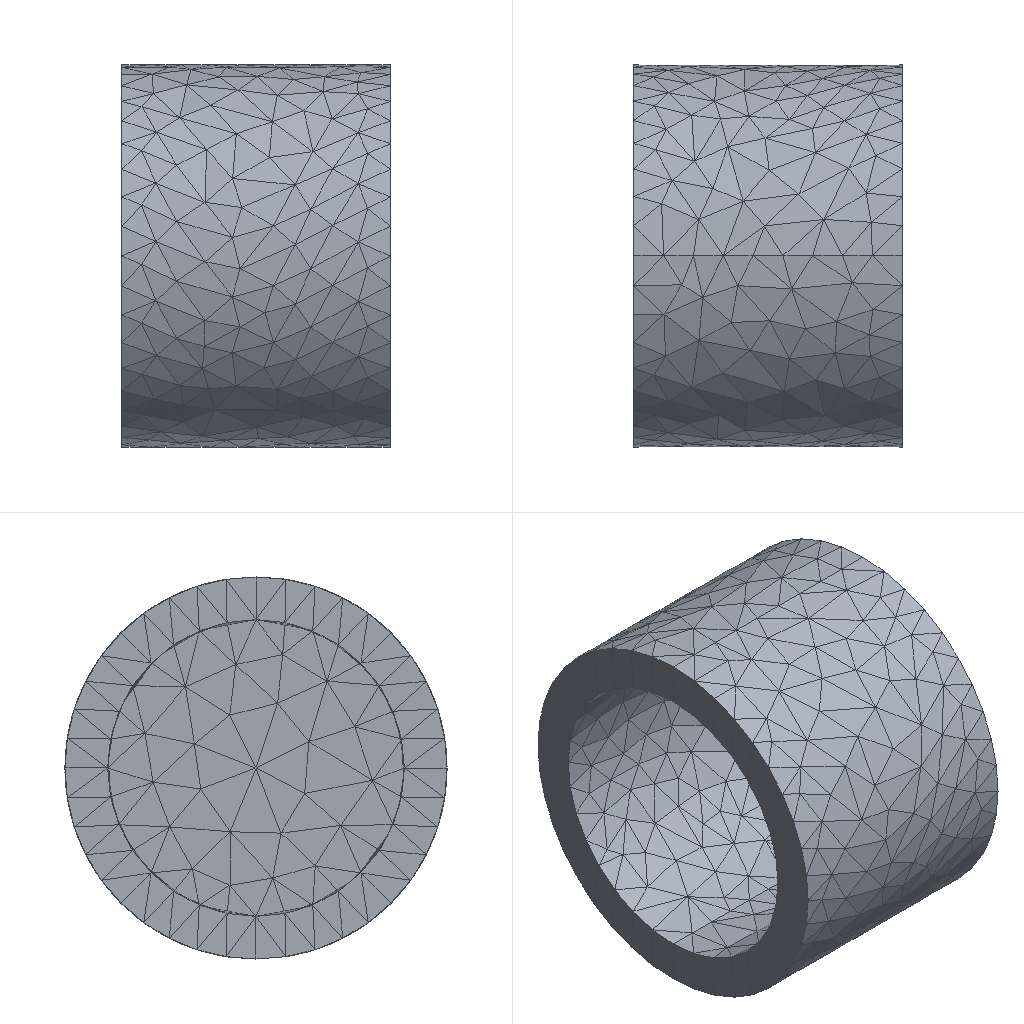Simulation study | ansys workbench
Ansys APDL input file, long lists of numbers shortened:
/batch
/config,noeldb,1     ! force off writing results to database
*get,_wallstrt,active,,time,wall
! ANSYS input file written by Workbench version 2022 R1
! File used for geometry attach:
/title,wbnew--____ (A5)
! ****** Begin Custom Load Command Snippet ******
/COM, ACT Extensions:
/COM,     LSDYNA, 2021.1
/COM,
! ****** End   Custom Load Command Snippet ******
*DIM,_wb_ProjectScratch_dir,string,248
_wb_ProjectScratch_dir(1) = ''
*DIM,_wb_SolverFiles_dir,string,248
_wb_SolverFiles_dir(1) = ''
*DIM,_wb_userfiles_dir,string,248
_wb_userfiles_dir(1) = ''
/com,--- Data in consistent NMM units. See Solving Units in the help system for more information.
/units,MPA
/nopr
/wb,file,start              !  signify a WB generated input file
/prep7
! Turn off shape checking because checks already performed inside WB mesher.
! See help system for more information.
SHPP,OFF,,NOWARN
/nolist
etcon,set             ! allow ANSYS to choose best KEYOP's for 180x elements, resets any applicable keyopt to MAPDL defaults
/com,*********** Nodes for the whole assembly ***********
nblock,3,,4614
(1i9,3e20.9e3)
        1     1.305000000E+03     0.000000000E+00     1.789968367E+02
! (4194 more lines like these left out)
-1
/wb,elem,start            !  set before creation of elements
/com,*********** Elements for Body 1 "__1-FreeParts|__-__1" ***********
et,1,187
eblock,19,solid,,2247
(19i9)
        1        1        1        1        0        0        0        0       10        0        1      105      684      200      612     1448     1992     1440     1445
! (4493 more lines like these left out)
-1
/wb,elem,end               !  done creating elements
/com,*********** Send User Defined Coordinate System(s) ***********
csys,0
toffst,273.15,  ! Temperature offset from absolute zero
/com,*********** Set Reference Temperature ***********
tref,22.
/wb,mat,start              !  starting to send materials
/com,*********** Send Materials ***********
Temperature = 'TEMP' ! Temperature
MP,DENS,1,7.85e-09,	! tonne mm^-3
MP,ALPX,1,1.2e-05,	! C^-1
MP,C,1,434000000,	! mm^2 s^-2 C^-1
MP,KXX,1,60.5,	! tonne mm s^-3 C^-1
MP,RSVX,1,0.00017,	! ohm mm
MP,EX,1,200000,	! tonne s^-2 mm^-1
MP,NUXY,1,0.3,
MP,MURX,1,10000,
/wb,mat,end                !  done sending materials
!************************* Model Summary ********************
!__1-FreeParts|__-__1,	结构钢,	matid,	1
!************************* End Model Summary ********************
! get the diagonal of the bounding box. Needed later for other things
*get,_xmin,node,,mnloc,x
*get,_ymin,node,,mnloc,y
*get,_zmin,node,,mnloc,z
*get,_xmax,node,,mxloc,x
*get,_ymax,node,,mxloc,y
*get,_zmax,node,,mxloc,z
_ASMDIAG=(_xmax-_xmin)*(_xmax-_xmin)+(_ymax-_ymin)*(_ymax-_ymin)+(_zmax-_zmin)*(_zmax-_zmin)
_ASMDIAG=SQRT(_ASMDIAG)
/wb,contact,start          !  starting to send contact
/wb,contact,end            !  done creating contacts
/golist
/wb,load,start             !  starting to send loads
/com,*********** Fixed Supports ***********
CMBLOCK,_FIXEDSU,NODE,      237
(8i10)
         1         2         3         4         5         6         7         8
! (29 more lines like these left out)
cmsel,s,_FIXEDSU
d,all,all
nsel,all
/com,*********** Define Pressure Using Surface Effect Elements "__" ***********
et,2,154
eblock,10,,,548
(15i9)
     3410        2        2        2        0       33       32      435      435      876      880      435      886
! (547 more lines like these left out)
-1
esel,s,type,,2
keyop,2,7,0                ! Use deformed area for application of load
esel,all
/com,*********** Define Pressure Using Surface Effect Elements "__ 2" ***********
et,3,154
eblock,10,,,368
(15i9)
     3958        3        3        3        0       67       66      388      388     1131     1134      388     1144
! (367 more lines like these left out)
-1
esel,s,type,,3
keyop,3,7,0                ! Use deformed area for application of load
esel,all
esel,all
/gst,on,on
fini
*get,_numnode,node,0,count
*get,_numelem,elem,0,count
*get, _MAXELEMNUM, elem, 0, NUM, MAX
*get, _MAXNODENUM, node, 0, NUM, MAX
*get, _MAXELEMTYPE, etyp, 0, NUM, MAX
*get, _MAXREALCONST, real, 0, NUM, MAX
/go
/wb,load,end               !  done creating loads
/com,--- Number of total nodes = %_numnode%
/com,--- Number of contact elements = 916
/com,--- Number of spring elements = 0
/com,--- Number of bearing elements = 0
/com,--- Number of solid elements = 2247
/com,--- Number of condensed parts = 0
/com,--- Number of total elements = %_numelem%
*get,_wallbsol,active,,time,wall
/com,****************************************************************************
/com,*************************    SOLUTION       ********************************
/com,****************************************************************************
/solu
antype,0                   ! static analysis
_thickRatio=  0     ! Ratio of thick parts in the model
eqsl,sparse,,,,,1
cntr,print,1               ! print out contact info and also make no initial contact an error
dmpoption,emat,no             ! Don't combine emat file for DANSYS
dmpoption,esav,no             ! Don't combine esav file for DANSYS
nldiag,cont,iter           ! print out contact info each equilibrium iteration
rescontrol,,none                 ! Do not keep any restart files
/com,****************************************************
/com,******************* SOLVE FOR LS 1 OF 1 ****************
esel,s,type,,2
nsle
sf,all,pres,20.
esel,s,type,,3
nsle
sf,all,pres,60.
nsel,all
esel,all
esel,all
/nopr
/gopr
nsub,1,1,1
time,1.
outres,erase
outres,all,none
outres,nsol,all,
outres,rsol,all
outres,eangl,all
outres,etmp,all
outres,veng,all
outres,strs,all,
outres,epel,all,
outres,eppl,all,
outres,cont,all,
! *********** WB SOLVE COMMAND ***********
! check interactive state
*get,ANSINTER_,active,,int
*if,ANSINTER_,ne,0,then
/eof
*endif
solve
/com *************** Write FE CONNECTORS *********
CEWRITE,file,ce,,INTE
/com,****************************************************
/com,*************** FINISHED SOLVE FOR LS 1 *************
*get,_wallasol,active,,time,wall
/nopr
*get,_numnode,node,0,count
*get,_numelem,elem,0,count
*get, _MAXELEMNUM, elem, 0, NUM, MAX
*get, _MAXNODENUM, node, 0, NUM, MAX,,,INTERNAL
*get, _MAXELEMTYPE, etyp, 0, NUM, MAX
*get, _MAXREALCONST, real, 0, NUM, MAX
/gopr
/post1
xmlo,ENCODING,ISO-8859-1
xmlo,parm
/xml,parm,xml
fini
/gopr
*get,_walldone,active,,time,wall
_preptime=(_wallbsol-_wallstrt)*3600
_solvtime=(_wallasol-_wallbsol)*3600
_posttime=(_walldone-_wallasol)*3600
_totaltim=(_walldone-_wallstrt)*3600
*get,_dlbratio,active,0,solu,dlbr
*get,_combtime,active,0,solu,comb
*get,_ssmode,active,0,solu,ssmm
*get,_ndofs,active,0,solu,ndof
*get,_sol_end_time,active,0,set,time
*if,_sol_end_time,eq,1.,then
/fclean				!clean distributed files
*endif
/com,--- Total number of nodes = %_numnode%
/com,--- Total number of elements = %_numelem%
/com,--- Element load balance ratio = %_dlbratio%
/com,--- Time to combine distributed files = %_combtime%
/com,--- Sparse memory mode = %_ssmode%
/com,--- Number of DOF = %_ndofs%
/wb,file,end               ! done with WB generated input